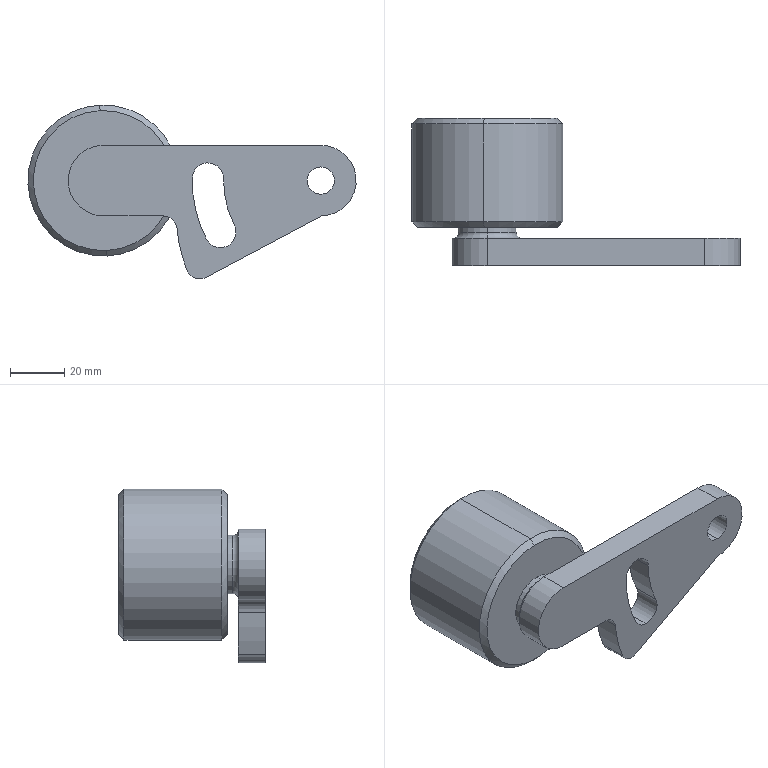Part | SolidWorks | features CompositeCurve 20 | 6 solids | 205 faces | box 120.656 x 54 x 63.864 mm | volume 111745 mm3 | cylinder 68 | torus 58 | plane 35 | sphere 32 | cone 12 | commonest cylinder face diameters 15 x6 10 x5 1.7 x4 2 x4 20.667 x4 26.333 x4